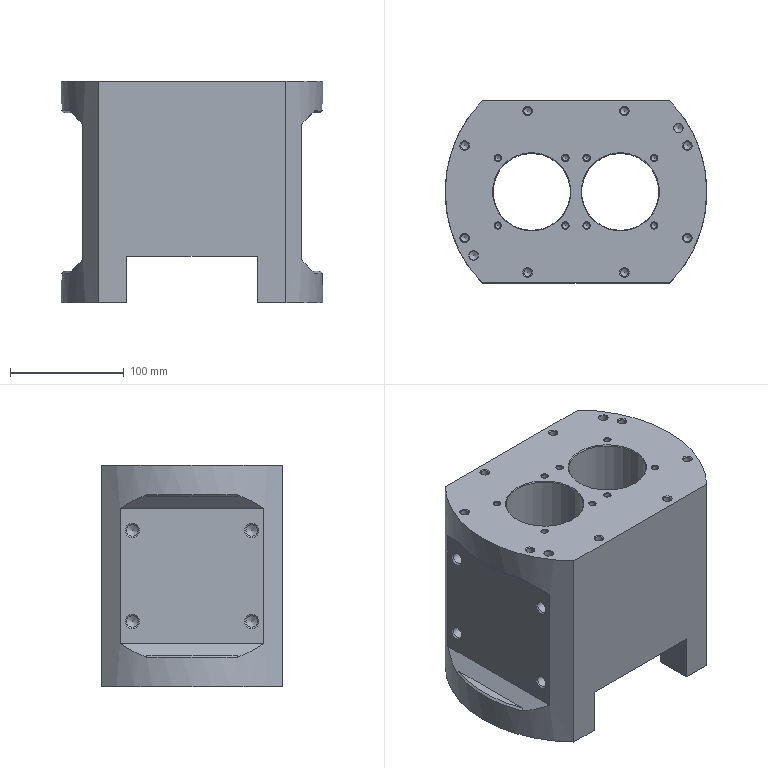NC program | NX | posted with a generic post | part box 230 x 160 x 195 mm
Lines 674 to 1584 of 6546:
(ZLEVEL_PROFILE_COPY , TOOL : D10)
N1340 T10 M6
N1342 G54
N1344 G17 G0 G90 X68.913 Y-34.137 B0. C0. S3500 M3
N1346 G43 Z30. H10
N1348 Z2.859
N1350 G94 G1 Z-0.141 F1000.
N1352 X70.004 Y-33.055
N1354 G3 X70.267 Y-32.09 R1.
N1356 G2 X66.273 Y-7.81 R129.993 F2200.
N1358 X68.051 Y22.092 R121.465
N1360 G1 X68.303 Y23.431
N1362 G2 X70.267 Y32.089 R133.086
N1364 G1 X70.265 Y32.27 Z-0.189
N1366 X70.267 Y32.449 Z-0.236
N1368 X70.272 Y32.628 Z-0.283
N1370 G3 X68.163 Y23.431 R133.781
N1372 G1 X67.911 Y22.092
N1374 G3 X66.131 Y-7.81 R121.38
N1376 X70.272 Y-32.628 R129.905
N1378 G1 X70.27 Y-32.808 Z-0.33
N1380 X70.272 Y-32.987 Z-0.377
N1382 X70.277 Y-33.165 Z-0.424
N1384 G2 X66.381 Y-12.366 R130.972
N1386 X67.074 Y17.919 R119.365
N1388 X70.277 Y33.166 R136.927
N1390 G1 X70.274 Y33.342 Z-0.471
N1392 X70.276 Y33.518 Z-0.519
N1394 X70.279 Y33.693 Z-0.566
N1396 G3 X67.971 Y23.877 R141.858
N1398 G1 X67.884 Y23.431
N1400 G3 X66.093 Y-10.934 R121.273
N1402 X70.279 Y-33.692 R132.524
N1404 G1 X70.281 Y-33.863 Z-0.613
N1406 X70.282 Y-34.033 Z-0.66
N1408 X70.287 Y-34.203 Z-0.707
N1410 G2 X65.995 Y-11.381 R132.113
N1412 X67.744 Y23.431 R121.1
N1414 G1 X67.832 Y23.877
N1416 G2 X70.287 Y34.203 R138.883
N1418 G1 X70.286 Y34.373 Z-0.754
N1420 X70.287 Y34.543 Z-0.801
N1422 X70.293 Y34.711 Z-0.849
N1424 G3 X67.692 Y23.877 R138.715
N1426 G1 X67.604 Y23.431
N1428 G3 X65.941 Y-12.273 R121.022
N1430 X70.293 Y-34.712 R132.842
N1432 G1 X70.29 Y-34.879 Z-0.896
N1434 X70.292 Y-35.044 Z-0.943
N1436 X70.299 Y-35.207 Z-0.99
N1438 G2 X66.233 Y-15.892 R133.312
N1440 X66.849 Y20.049 R119.865
N1442 X70.299 Y35.207 R138.502
N1444 G1 X70.297 Y35.371 Z-1.037
N1446 X70.298 Y35.534 Z-1.084
N1448 X70.305 Y35.695 Z-1.131
N1450 G3 X67.413 Y23.877 R138.622
N1452 G1 X67.324 Y23.431
N1454 G3 X65.66 Y-12.273 R120.9
N1456 X70.305 Y-35.695 R132.646
N1458 G1 X70.302 Y-35.859 Z-1.179
N1460 X70.304 Y-36.022 Z-1.226
N1462 X70.31 Y-36.183 Z-1.273
N1464 G2 X65.771 Y-14.505 R134.113
N1466 X67.184 Y23.431 R120.734
N1468 G1 X67.273 Y23.877
N1470 G2 X70.31 Y36.184 R140.183
N1472 G1 X70.306 Y36.346 Z-1.32
N1474 X70.307 Y36.506 Z-1.367
N1476 X70.315 Y36.665 Z-1.414
N1478 G3 X67.134 Y23.877 R141.731
N1480 G1 X67.044 Y23.431
N1482 G3 X65.74 Y-15.397 R120.755
N1484 X70.315 Y-36.664 R135.262
N1486 G1 X70.313 Y-36.822 Z-1.461
N1488 X70.315 Y-36.98 Z-1.509
N1490 X70.321 Y-37.135 Z-1.556
N1492 G2 X65.6 Y-15.397 R135.399
N1494 X66.651 Y22.092 R120.306
N1496 X70.32 Y37.136 R140.552
N1498 G1 X70.319 Y37.293 Z-1.603
N1500 X70.321 Y37.449 Z-1.65
N1502 X70.326 Y37.604 Z-1.697
N1504 G3 X66.68 Y22.984 R141.925
N1506 X65.46 Y-15.397 R120.284
N1508 X70.326 Y-37.604 R135.836
N1510 G1 X70.324 Y-37.759 Z-1.744
N1512 X70.326 Y-37.913 Z-1.791
N1514 X70.332 Y-38.066 Z-1.839
N1516 G2 X65.908 Y-19.414 R138.626
N1518 X64.474 Y-6.025 R118.166
N1520 X64.4 Y-3.039 R60.156
N1522 G1 Y2.959
N1524 G2 X64.526 Y6.868 R60.811
N1526 G1 X64.644 Y8.703
N1528 X64.674 Y9.149
N1530 G2 X68.118 Y30.125 R126.73
N1532 G1 X68.344 Y31.018
N1534 G2 X70.332 Y38.065 R142.346
N1536 G1 X70.331 Y38.218 Z-1.886
N1538 X70.334 Y38.37 Z-1.933
N1540 X70.338 Y38.521 Z-1.98
N1542 G3 X68.321 Y31.464 R141.46
N1544 G1 X68.206 Y31.018
N1546 G3 X64.533 Y9.149 R127.197
N1548 X64.4 Y6.385 R42.783
N1550 G1 Y-6.39
N1552 G3 X64.48 Y-8.386 R34.933
N1554 X65.768 Y-19.414 R116.791
N1556 X70.339 Y-38.52 R138.489
N1558 G1 Y-38.672 Z-2.028
N1560 X70.341 Y-38.824 Z-2.075
N1562 X70.346 Y-38.974 Z-2.122
N1564 G2 X65.702 Y-19.86 R139.282
N1566 X64.433 Y-9.595 R115.739
N1568 G1 X64.401 Y-8.703
N1570 X64.4 Y-8.533
N1572 Y8.538
N1574 X64.401 Y8.703
N1576 X64.433 Y9.595
N1578 G2 X68.067 Y31.018 R126.18
N1580 G1 X68.184 Y31.464
N1582 G2 X70.345 Y38.976 R147.744
N1584 G1 Y39.129 Z-2.169
N1586 X70.347 Y39.281 Z-2.217
N1588 X70.352 Y39.432 Z-2.264
N1590 G3 X68.522 Y33.249 R155.693
N1592 G1 X68.4 Y32.803
N1594 G3 X64.533 Y12.273 R129.403
N1596 X64.4 Y10.22 R21.989
N1598 G1 Y-10.223
N1600 G3 X64.477 Y-11.687 R17.623
N1602 X65.343 Y-18.521 R108.629
N1604 X70.353 Y-39.429 R139.073
N1606 G1 X70.352 Y-39.58 Z-2.312
N1608 X70.355 Y-39.731 Z-2.359
N1610 X70.36 Y-39.881 Z-2.406
N1612 G2 X65.897 Y-22.538 R143.324
N1614 X64.446 Y-12.719 R116.396
N1616 X64.4 Y-11.707 R14.603
N1618 G1 Y11.702
N1620 G2 X64.466 Y12.906 R10.992
N1622 X67.931 Y31.563 R128.608
N1624 X70.359 Y39.886 R164.25
N1626 G1 Y40.037 Z-2.454
N1628 X70.362 Y40.187 Z-2.501
N1630 X70.367 Y40.337 Z-2.549
N1632 G3 X68.621 Y34.588 R175.228
N1634 G1 X68.494 Y34.142
N1636 G3 X64.616 Y15.397 R131.517
N1638 G1 X64.561 Y14.951
N1640 X64.472 Y14.179
N1642 G3 X64.4 Y13.001 R11.826
N1644 G1 Y-12.998
N1646 G3 X64.486 Y-14.327 R12.592
N1648 X65.928 Y-23.431 R115.814
N1650 X70.369 Y-40.33 R145.407
N1652 G1 Y-40.482 Z-2.596
N1654 X70.372 Y-40.632 Z-2.644
N1656 X70.377 Y-40.781 Z-2.691
N1658 G2 X66.057 Y-24.769 R149.788
N1660 X64.475 Y-15.397 R130.935
N1662 X64.4 Y-14.176 R10.242
N1664 G1 Y14.18
N1666 G2 X64.475 Y15.397 R10.235
N1668 X68.871 Y35.927 R132.708
N1670 G1 X69.002 Y36.373
N1672 X70.246 Y40.39
N1674 X70.375 Y40.79
N1676 X70.376 Y40.947 Z-2.739
N1678 X70.379 Y41.104 Z-2.787
N1680 X70.383 Y41.26 Z-2.834
N1682 G3 X68.367 Y34.657 R234.287
N1684 X64.48 Y16.428 R129.606
N1686 X64.4 Y15.267 R8.433
N1688 G1 Y-15.269
N1690 G3 X64.479 Y-16.414 R8.376
N1692 X67.373 Y-31.018 R127.116
N1694 X70.387 Y-41.249 R177.576
N1696 G1 X70.388 Y-41.407 Z-2.882
N1698 X70.392 Y-41.564 Z-2.929
N1700 X70.396 Y-41.721 Z-2.977
N1702 G2 X68.209 Y-34.588 R250.981
N1704 X64.581 Y-18.138 R132.255
N1706 G1 X64.509 Y-17.629
N1708 G2 X64.4 Y-16.281 R9.712
N1710 G1 Y16.278
N1712 G2 X64.509 Y17.629 R9.699
N1714 G1 X64.581 Y18.136
N1716 G2 X68.73 Y36.373 R134.02
N1718 G1 X68.998 Y37.266
N1720 X70.253 Y41.282
N1722 X70.392 Y41.733
N1724 X70.329 Y41.761 Z-3.049
N1726 X70.249 Y41.798 Z-3.12
N1728 G2 X70.122 Y41.283 R4.325
N1730 G1 X68.862 Y37.266
N1732 X68.593 Y36.373
N1734 G3 X64.5 Y18.521 R133.997
N1736 X64.4 Y17.233 R8.601
N1738 G1 Y-17.237
N1740 G3 X64.5 Y-18.521 R8.595
N1742 X66.326 Y-27.894 R132.186
N1744 X70.067 Y-41.09 R159.82
N1746 G2 X70.245 Y-41.805 R4.982
N1748 G1 X70.142 Y-41.745 Z-3.192
N1750 X70.058 Y-41.683 Z-3.263
N1752 G3 X70.02 Y-41.389 R0.813
N1754 G2 X67.665 Y-33.637 R209.296
N1756 X64.508 Y-19.412 R127.619
N1758 X64.4 Y-18.142 R8.332
N1760 G1 Y18.139
N1762 G2 X64.508 Y19.414 R8.331
N1764 X68.456 Y36.373 R132.204
N1766 G1 X68.725 Y37.266
N1768 X70.017 Y41.386
N1770 G3 X70.06 Y41.694 R0.952
N1772 G1 X70.032 Y41.864 Z-3.299
N1774 X69.998 Y42.034 Z-3.335
N1776 X69.974 Y42.203 Z-3.371
N1778 X69.95 Y42.373 Z-3.407
N1780 G3 X69.904 Y41.506 R6.558
N1782 G1 X69.85 Y41.282
N1784 X69.145 Y39.051
N1786 X69.006 Y38.605
N1788 X68.727 Y37.712
N1790 G3 X64.665 Y21.199 R136.391
N1792 G1 X64.516 Y20.307
N1794 G3 X64.4 Y18.968 R8.213
N1796 G1 Y-18.968
N1798 G3 X64.516 Y-20.307 R8.213
N1800 G1 X64.665 Y-21.199
N1802 G3 X68.846 Y-38.106 R137.693
N1804 G1 X69.849 Y-41.282
N1806 X69.904 Y-41.506
N1808 G3 X69.947 Y-42.376 R5.8
N1810 G1 X69.866 Y-42.518 Z-3.479
N1812 X69.794 Y-42.658 Z-3.55
N1814 X69.789 Y-42.621
N1816 X69.76 Y-41.506
N1818 X69.712 Y-41.282
N1820 X68.479 Y-37.331
N1822 G2 X65.703 Y-27.001 R134.232
N1824 X64.532 Y-21.24 R132.357
N1826 X64.4 Y-19.826 R8.335
N1828 G1 Y19.825
N1830 G2 X64.538 Y21.282 R8.569
N1832 X68.696 Y38.055 R137.191
N1834 G1 X69.723 Y41.305
N1836 X69.756 Y41.399
N1838 Y41.499
N1840 X69.797 Y42.655
N1842 X69.721 Y42.793 Z-3.622
N1844 X69.655 Y42.931 Z-3.693
N1846 X69.62 Y41.541
N1848 G2 X69.571 Y41.246 R1.058
N1850 G1 X68.872 Y39.051
N1852 X68.328 Y37.303
N1854 G3 X64.533 Y21.989 R133.678
N1856 X64.4 Y20.614 R7.933
N1858 G1 Y-20.614
N1860 G3 X64.529 Y-21.966 R7.931
N1862 X66.732 Y-31.746 R123.326
N1864 X69.533 Y-41.126 R175.566
N1866 G2 X69.616 Y-41.607 R1.674
N1868 G1 X69.65 Y-42.936
N1870 X69.571 Y-43.071 Z-3.765
N1872 X69.506 Y-43.205 Z-3.836
N1874 G3 X69.443 Y-41.282 R34.087
N1876 G2 X67.162 Y-33.815 R211.646
N1878 X64.536 Y-22.731 R125.863
N1880 X64.4 Y-21.354 R7.816
N1882 G1 Y21.353
N1884 G2 X64.55 Y22.799 R7.816
N1886 X68.041 Y36.82 R132.86
N1888 G1 X68.177 Y37.266
N1890 X69.164 Y40.39
N1892 X69.439 Y41.254
N1894 G3 X69.478 Y41.493 R0.837
N1896 G1 X69.504 Y43.068
N1898 X69.512 Y43.2
N1900 X69.433 Y43.332 Z-3.907
N1902 X69.366 Y43.463 Z-3.979
N1904 X69.334 Y41.473
N1906 X69.338 Y41.376
N1908 X69.313 Y41.282
N1910 X68.245 Y37.91
N1912 G3 X64.578 Y23.68 R134.741
N1914 X64.4 Y22.092 R9.31
N1916 G1 Y-22.092
N1918 G3 X64.567 Y-23.624 R8.839
N1920 X67.308 Y-34.803 R129.797
N1922 X69.308 Y-41.282 R230.906
N1924 G2 X69.359 Y-43.47 R51.569
N1926 G1 X69.286 Y-43.608 Z-4.05
N1928 X69.221 Y-43.747 Z-4.121
N1930 X69.215 Y-43.514
N1932 X69.192 Y-41.506
N1934 X69.173 Y-41.282
N1936 G2 X67.249 Y-35.071 R238.178
N1938 X64.535 Y-24.155 R130.185
N1940 X64.4 Y-22.808 R6.766
N1942 G1 Y22.805
N1944 G2 X64.541 Y24.194 R6.911
N1946 X68.123 Y37.954 R135.777
N1948 G1 X69.179 Y41.282
N1950 X69.196 Y41.506
N1952 X69.222 Y43.514
N1954 X69.228 Y43.738
N1956 X69.157 Y43.897 Z-4.191
N1958 X69.089 Y44.055 Z-4.262
N1960 X69.086 Y43.96
N1962 X69.056 Y41.506
N1964 X69.044 Y41.282
N1966 X67.968 Y37.89
N1968 G3 X64.54 Y24.839 R133.943
N1970 X64.4 Y23.484 R6.611
N1972 G1 Y-23.486
N1974 G3 X64.538 Y-24.829 R6.594
N1976 X67.047 Y-34.845 R127.775
N1978 X69.038 Y-41.282 R236.882
N1980 G1 X69.051 Y-41.506
N1982 X69.079 Y-43.96
N1984 X69.082 Y-44.064
N1986 X69.011 Y-44.243 Z-4.333
N1988 X68.943 Y-44.421 Z-4.404
N1990 X68.939 Y-43.96
N1992 X68.91 Y-41.506
N1994 X68.903 Y-41.282
N1996 G2 X67.347 Y-36.315 R363.413
N1998 X64.559 Y-25.562 R129.331
N2000 X64.4 Y-24.137 R7.216
N2002 G1 Y24.138
N2004 G2 X64.561 Y25.571 R7.217
N2006 X67.954 Y38.286 R134.904
N2008 G1 X68.813 Y40.974
N2010 X68.909 Y41.282
N2012 X68.916 Y41.506
N2014 X68.945 Y43.96
N2016 X68.948 Y44.414
N2018 X68.878 Y44.594 Z-4.474
N2020 X68.809 Y44.773 Z-4.545
N2022 X68.807 Y44.407
N2024 X68.773 Y41.282
N2026 X68.637 Y40.836
N2028 X67.774 Y38.149
N2030 G3 X64.541 Y26.108 R128.966
N2032 X64.4 Y24.769 R7.655
N2034 G1 Y-24.769
N2036 G3 X64.569 Y-26.239 R7.46
N2038 G1 X64.735 Y-27.001
N2040 G3 X67.36 Y-36.82 R137.507
N2042 G1 X67.499 Y-37.266
N2044 X68.632 Y-40.836
N2046 X68.767 Y-41.282
N2048 X68.805 Y-44.778
N2050 X68.736 Y-44.955 Z-4.616
N2052 X68.67 Y-45.132 Z-4.686
N2054 X68.626 Y-41.282
N2056 X68.498 Y-40.836
N2058 X67.784 Y-38.605
N2060 G2 X64.598 Y-27.001 R139.858
N2062 X64.4 Y-25.401 R7.301
N2064 G1 Y25.399
N2066 G2 X64.598 Y27.001 R7.299
N2068 X67.922 Y39.028 R139.65
N2070 G1 X68.504 Y40.836
N2072 X68.633 Y41.282
N2074 X68.673 Y45.129
N2076 X68.599 Y45.305 Z-4.757
N2078 X68.533 Y45.481 Z-4.828
N2080 X68.493 Y41.282
N2082 G2 X68.335 Y40.724 R7.93
N2084 G1 X67.922 Y39.443
N2086 G3 X64.561 Y27.447 R141.207
N2088 X64.4 Y26.006 R6.468
N2090 G1 Y-26.006
N2092 G3 X64.569 Y-27.482 R6.465
N2094 X67.725 Y-38.848 R142.365
N2096 G1 X68.293 Y-40.606
N2098 G2 X68.486 Y-41.282 R10.277
N2100 G1 X68.531 Y-45.483
N2102 X68.456 Y-45.657 Z-4.899
N2104 X68.389 Y-45.831 Z-4.969
N2106 X68.346 Y-41.282
N2108 X68.302 Y-41.059
N2110 X67.359 Y-38.109
N2112 G2 X64.585 Y-28.109 R134.184
N2114 X64.4 Y-26.598 R6.925
N2116 G1 Y26.6
N2118 G2 X64.578 Y28.081 R6.924
N2120 X68.096 Y40.39 R141.405
N2122 G1 X68.325 Y41.106
N2124 X68.355 Y41.192
N2126 X68.353 Y41.282
N2128 X68.39 Y45.83
N2130 X68.317 Y46.004 Z-5.04
N2132 X68.247 Y46.178 Z-5.111
N2134 X68.213 Y41.308
N2136 G2 X68.169 Y41.031 R0.928
N2138 G1 X67.963 Y40.39
N2140 G3 X64.578 Y28.644 R139.644
N2142 X64.4 Y27.176 R6.636
N2144 G1 Y-27.169
N2146 G3 X64.578 Y-28.644 R6.635
N2148 X68.039 Y-40.646 R145.378
N2150 G2 X68.207 Y-41.282 R4.919
N2152 X68.246 Y-46.179 R255.457
N2154 G1 X68.175 Y-46.353 Z-5.181
N2156 X68.11 Y-46.526 Z-5.252
N2158 G3 X68.067 Y-41.282 R363.385
N2160 G1 X68.033 Y-41.059
N2162 G2 X65.393 Y-32.357 R174.697
N2164 X64.578 Y-29.206 R94.72
N2166 X64.4 Y-27.743 R6.759
N2168 G1 Y27.744
N2170 G2 X64.578 Y29.206 R6.759
N2172 X68. Y40.904 R141.457
N2174 G3 X68.073 Y41.337 R1.376
N2176 G1 X68.111 Y46.526
N2178 X68.035 Y46.696 Z-5.323
N2180 X67.969 Y46.866 Z-5.394
N2182 X67.943 Y42.175
N2184 X67.932 Y41.244
N2186 G2 X67.883 Y40.96 R0.919
N2188 G3 X64.624 Y29.964 R148.891
N2190 X64.4 Y28.297 R7.242
N2192 G1 Y-28.297
N2194 G3 X64.618 Y-29.941 R7.175
N2196 X66.848 Y-37.768 R135.985
N2198 G1 X67.922 Y-41.149
N2200 G2 X67.968 Y-46.866 R278.812
N2202 G1 X67.893 Y-47.035 Z-5.464
N2204 X67.827 Y-47.203 Z-5.535
N2206 G3 X67.791 Y-41.251 R423.014
N2208 X67.747 Y-40.994 R0.847
N2210 G2 X64.578 Y-30.319 R161.459
N2212 X64.4 Y-28.841 R6.285
N2214 G1 Y28.838
N2216 G2 X64.578 Y30.319 R6.283
N2218 X67.778 Y41.059 R153.85
N2220 G1 X67.793 Y41.282
N2222 X67.823 Y46.638
N2224 X67.827 Y47.202
N2226 X67.752 Y47.37 Z-5.606
N2228 X67.682 Y47.539 Z-5.676
N2230 Y46.638
N2232 X67.654 Y41.282
N2234 X67.645 Y41.059
N2236 G3 X64.578 Y30.83 R153.623
N2238 X64.4 Y29.373 R6.519
N2240 G1 Y-29.37
N2242 G3 X64.578 Y-30.83 R6.518
N2244 X67.619 Y-41.011 R160.641
N2246 G2 X67.653 Y-41.212 R0.659
N2248 X67.682 Y-47.539 R419.652
N2250 G1 X67.611 Y-47.707 Z-5.747
N2252 X67.544 Y-47.876 Z-5.818
N2254 X67.531 Y-42.621
N2256 X67.516 Y-41.282
N2258 X67.502 Y-41.059
N2260 G2 X64.612 Y-31.464 R158.472
N2262 X64.4 Y-29.881 R6.343
N2264 G1 Y29.881
N2266 G2 X64.612 Y31.464 R6.343
N2268 X67.511 Y41.059 R151.278
N2270 G3 X67.544 Y47.875 R594.075
N2272 G1 X67.47 Y48.041 Z-5.889
N2274 X67.403 Y48.206 Z-5.959
N2276 X67.384 Y42.175
N2278 X67.373 Y41.059
N2280 X67.162 Y40.39
N2282 G3 X64.596 Y31.91 R136.704
N2284 X64.4 Y30.405 R6.491
N2286 G1 Y-30.405
N2288 G3 X64.596 Y-31.91 R6.492
N2290 X67.368 Y-41.059 R160.295
N2292 G1 X67.379 Y-41.282
N2294 X67.403 Y-48.206
N2296 X67.328 Y-48.369 Z-6.03
N2298 X67.261 Y-48.531 Z-6.101
N2300 X67.246 Y-41.729
N2302 X67.234 Y-41.059
N2304 G2 X64.699 Y-32.803 R175.194
N2306 G1 X64.578 Y-32.35
N2308 G2 X64.4 Y-30.906 R6.61
N2310 G1 Y30.906
N2312 G2 X64.578 Y32.35 R6.61
N2314 G1 X64.699 Y32.803
N2316 G2 X67.179 Y40.836 R144.311
N2318 G1 X67.234 Y41.059
N2320 X67.244 Y42.175
N2322 X67.261 Y48.531
N2324 X67.187 Y48.693 Z-6.171
N2326 X67.117 Y48.856 Z-6.242
N2328 X67.105 Y42.175
N2330 X67.094 Y41.059
N2332 X67.046 Y40.836
N2334 G3 X64.684 Y33.249 R149.366
N2336 X64.4 Y31.401 R6.721
N2338 G1 Y-31.403
N2340 G3 X64.684 Y-33.249 R6.723
N2342 X67.1 Y-41.059 R192.176
N2344 G1 X67.108 Y-41.729
N2346 X67.117 Y-48.856
N2348 X67.046 Y-49.018 Z-6.313
N2350 X66.977 Y-49.181 Z-6.384
N2352 X66.969 Y-41.729
N2354 X66.964 Y-41.059
N2356 X66.904 Y-40.836
N2358 X66.607 Y-39.944
N2360 G2 X64.624 Y-33.501 R150.722
N2362 X64.4 Y-31.89 R5.908
N2364 G1 Y31.89
N2366 G2 X64.622 Y33.495 R5.902
N2368 X66.912 Y40.836 R142.669
N2370 G1 X66.955 Y41.059
N2372 X66.965 Y42.175
N2374 X66.977 Y49.18
N2376 X66.904 Y49.341 Z-6.454
N2378 X66.84 Y49.501 Z-6.525
N2380 X66.834 Y49.316
N2382 X66.821 Y41.207
N2384 G2 X66.778 Y40.836 R1.645
N2386 G3 X64.661 Y34.112 R143.8
N2388 X64.4 Y32.357 R6.68
N2390 G1 Y-32.357
N2392 G3 X64.578 Y-33.798 R6.667
N2394 X66.691 Y-40.584 R137.913
N2396 G2 X66.825 Y-41.059 R4.753
N2398 G1 X66.84 Y-49.501
N2400 X66.763 Y-49.66 Z-6.596
N2402 X66.695 Y-49.819 Z-6.666
N2404 X66.687 Y-41.103
N2406 G3 X66.642 Y-40.831 R0.84
N2408 G2 X64.671 Y-34.588 R136.317
N2410 X64.4 Y-32.834 R6.319
N2412 G1 Y32.835
N2414 G2 X64.671 Y34.588 R6.318
N2416 X66.645 Y40.836 R133.395
N2418 G3 X66.682 Y41.177 R1.599
N2420 G1 X66.695 Y49.819
N2422 X66.621 Y49.976 Z-6.737
N2424 X66.552 Y50.132 Z-6.808
N2426 X66.537 Y40.943
N2428 X66.526 Y40.889
N2430 G3 X64.667 Y35.034 R137.959
N2432 X64.4 Y33.297 R6.318
N2434 G1 Y-33.298
N2436 G3 X64.667 Y-35.034 R6.318
N2438 X66.541 Y-40.941 R146.081
N2440 G1 X66.548 Y-41.
N2442 X66.552 Y-50.132
N2444 X66.48 Y-50.289 Z-6.879
N2446 X66.415 Y-50.446 Z-6.949
N2448 X66.409 Y-50.208
N2450 X66.405 Y-40.971
N2452 X66.402 Y-40.915
N2454 G2 X64.663 Y-35.481 R148.465
N2456 X64.4 Y-33.753 R6.314
N2458 G1 Y33.755
N2460 G2 X64.663 Y35.481 R6.314
N2462 X66.396 Y40.917 R172.222
N2464 G1 X66.403 Y41.729
N2466 X66.409 Y50.208
N2468 X66.415 Y50.446
N2470 X66.339 Y50.602 Z-7.02
N2472 X66.272 Y50.758 Z-7.091
N2474 X66.263 Y41.729
N2476 X66.26 Y40.946
N2478 X66.245 Y40.836
N2480 G3 X64.659 Y35.927 R148.881
N2482 X64.4 Y34.202 R6.309
N2484 G1 Y-34.202
N2486 G3 X64.659 Y-35.927 R6.309
N2488 X66.094 Y-40.39 R143.354
N2490 G1 X66.245 Y-40.836
N2492 X66.266 Y-40.945
N2494 X66.268 Y-50.655
N2496 X66.271 Y-50.758
N2498 X66.197 Y-50.913 Z-7.161
N2500 X66.127 Y-51.068 Z-7.232
N2502 X66.125 Y-41.282
N2504 X66.124 Y-40.919
N2506 X66.112 Y-40.836
N2508 G2 X64.661 Y-36.373 R149.181
N2510 X64.4 Y-34.646 R5.989
N2512 G1 Y34.647
N2514 G2 X64.661 Y36.373 R5.989
N2516 X66.112 Y40.836 R149.18
N2518 G1 X66.121 Y40.924
N2520 X66.127 Y51.068
N2522 X66.056 Y51.22 Z-7.303
N2524 X65.99 Y51.371 Z-7.373
N2526 X65.979 Y40.836
N2528 G3 X64.669 Y36.82 R133.798
N2530 X64.4 Y35.081 R6.086
N2532 G1 Y-35.082
N2534 G3 X64.669 Y-36.82 R6.088
N2536 X65.979 Y-40.836 R132.601
N2538 G1 X65.99 Y-51.371
N2540 X65.914 Y-51.523 Z-7.444
N2542 X65.847 Y-51.674 Z-7.515
N2544 X65.844 Y-51.547
N2546 Y-41.074
N2548 Y-40.826
N2550 G2 X64.677 Y-37.266 R116.391
N2552 X64.4 Y-35.513 R6.095
N2554 G1 Y35.515
N2556 G2 X64.677 Y37.266 R6.097
N2558 X65.844 Y40.818 R104.557
N2560 G1 Y41.073
N2562 X65.841 Y42.175
N2564 X65.844 Y51.547
N2566 X65.847 Y51.674
N2568 X65.773 Y51.826 Z-7.586
N2570 X65.703 Y51.977 Z-7.656
N2572 X65.701 Y42.175
N2574 X65.702 Y41.443
N2576 Y40.801
N2578 G3 X64.685 Y37.712 R102.699
N2580 X64.4 Y35.927 R6.081
N2582 G1 Y-35.927
N2584 G3 X64.685 Y-37.712 R6.081
N2586 X65.702 Y-40.801 R102.75
N2588 G1 Y-41.443
N2590 X65.703 Y-51.977
N2592 X65.632 Y-52.128 Z-7.727
N2594 X65.565 Y-52.279 Z-7.798
N2596 X65.561 Y-51.994
N2598 X65.559 Y-41.809
N2600 X65.561 Y-41.729
N2602 Y-40.783
N2604 X64.835 Y-38.605
N2606 X64.693 Y-38.158
N2608 G2 X64.4 Y-36.358 R6.096
N2610 G1 Y36.359
N2612 G2 X64.693 Y38.158 R6.098
N2614 G1 X64.835 Y38.605
N2616 X65.561 Y40.783
N2618 Y41.729
N2620 X65.559 Y41.809
N2622 X65.561 Y51.994
N2624 X65.565 Y52.278
N2626 X65.49 Y52.427 Z-7.868
N2628 X65.423 Y52.576 Z-7.939
N2630 X65.419 Y52.44
N2632 Y41.729
N2634 Y40.757
N2636 X64.701 Y38.605
N2638 G3 X64.4 Y36.771 R6.061
N2640 G1 Y-36.771
N2642 G3 X64.701 Y-38.605 R6.061
N2644 G1 X65.419 Y-40.757
N2646 Y-41.729
N2648 Y-52.44
N2650 X65.423 Y-52.576
N2652 X65.349 Y-52.722 Z-8.01
N2654 X65.279 Y-52.869 Z-8.081
N2656 X65.278 Y-42.524
N2658 Y-40.731
N2660 G2 X64.578 Y-38.609 R31.247
N2662 X64.4 Y-37.181 R6.257
N2664 G1 Y37.182
N2666 G2 X64.578 Y38.609 R6.258
N2668 X65.278 Y40.731 R31.247
N2670 G1 Y42.524
N2672 X65.279 Y52.869
N2674 X65.207 Y53.015 Z-8.151
N2676 X65.14 Y53.162 Z-8.222
N2678 X65.137 Y52.886
N2680 X65.135 Y42.879
N2682 X65.137 Y42.621
N2684 X65.136 Y40.694
N2686 X64.729 Y39.497
N2688 G3 X64.4 Y37.584 R5.738
N2690 G1 Y-37.584
N2692 G3 X64.729 Y-39.497 R5.738
N2694 G1 X65.136 Y-40.694
N2696 X65.137 Y-42.621
N2698 Y-52.886
N2700 X65.14 Y-53.162
N2702 X65.066 Y-53.308 Z-8.293
N2704 X64.998 Y-53.454 Z-8.363
N2706 X64.995 Y-53.333
N2708 Y-43.068
N2710 Y-40.679
N2712 X64.578 Y-39.395
N2714 G2 X64.4 Y-37.984 R6.257
N2716 G1 Y37.985
N2718 G2 X64.578 Y39.395 R6.257
N2720 G1 X64.995 Y40.679
N2722 Y43.068
N2724 Y53.333
N2726 X64.998 Y53.454
N2728 X64.924 Y53.601 Z-8.434
N2730 X64.855 Y53.747 Z-8.505
N2732 X64.854 Y43.514
N2734 Y40.653
N2736 X64.625 Y39.944
N2738 G3 X64.4 Y38.392 R5.46
N2740 G1 Y-38.379
N2742 G3 X64.656 Y-40.03 R5.454
N2744 G1 X64.854 Y-40.653
N2746 Y-43.514
N2748 X64.855 Y-53.747
N2750 X64.783 Y-53.89 Z-8.576
N2752 X64.716 Y-54.032 Z-8.646
N2754 X64.712 Y-53.779
N2756 Y-43.92
N2758 Y-40.619
N2760 G2 X64.4 Y-38.769 R5.978
N2762 G1 Y38.769
N2764 G2 X64.712 Y40.619 R5.978
N2766 G1 Y43.92
N2768 Y53.779
N2770 X64.716 Y54.032
N2772 X64.642 Y54.174 Z-8.717
N2774 X64.574 Y54.316 Z-8.788
N2776 X64.571 Y54.225
N2778 Y43.96
N2780 Y40.543
N2782 G3 X64.4 Y39.154 R6.444
N2784 G1 Y-39.154
N2786 G3 X64.571 Y-40.543 R6.444
N2788 G1 Y-43.96
N2790 Y-54.225
N2792 X64.574 Y-54.316
N2794 X64.5 Y-54.457 Z-8.858
N2796 X64.432 Y-54.599 Z-8.929
N2798 X64.429 Y-44.407
N2800 Y-40.145
N2802 X64.4 Y-39.536
N2804 Y39.536
N2806 X64.429 Y40.145
N2808 Y44.407
N2810 X64.432 Y54.599
N2812 X64.359 Y54.741 Z-9.
N2814 X64.292 Y54.882 Z-9.071
N2816 X64.288 Y54.671
N2818 Y44.853
N2820 Y-44.853
N2822 Y-54.671
N2824 X64.292 Y-54.882
N2826 X64.217 Y-55.023 Z-9.141
N2828 X64.148 Y-55.164 Z-9.212
N2830 X64.147 Y-55.118
N2832 Y-45.266
N2834 Y45.266
N2836 Y55.118
N2838 X64.148 Y55.164
N2840 X64.076 Y55.302 Z-9.283
N2842 X64.008 Y55.441 Z-9.353
N2844 X64.005 Y55.118
N2846 Y45.299
N2848 Y-45.299
N2850 Y-55.118
N2852 X64.008 Y-55.441
N2854 X63.934 Y-55.578 Z-9.424
N2856 X63.867 Y-55.716 Z-9.495
N2858 X63.864 Y-55.564
N2860 Y-45.745
N2862 Y45.745
N2864 Y55.564
N2866 X63.867 Y55.716
N2868 X63.793 Y55.853 Z-9.566
N2870 X63.723 Y55.99 Z-9.636
N2872 X63.722 Y46.192
N2874 Y-46.192
N2876 X63.723 Y-55.99
N2878 X63.652 Y-56.127 Z-9.707
N2880 X63.585 Y-56.264 Z-9.778
N2882 X63.581 Y-56.01
N2884 Y-46.192
N2886 Y56.01
N2888 X63.585 Y56.264
N2890 X63.51 Y56.401 Z-9.848
N2892 X63.442 Y56.538 Z-9.919
N2894 X63.439 Y56.457
N2896 X63.438 Y46.883
N2898 X63.439 Y46.638
N2900 Y-46.638
N2902 X63.438 Y-46.883
N2904 X63.439 Y-56.457
N2906 X63.442 Y-56.538
N2908 X63.369 Y-56.672 Z-9.99
N2910 X63.301 Y-56.806 Z-10.061
N2912 X63.298 Y-56.457
N2914 Y56.457
N2916 X63.301 Y56.806
N2918 X63.227 Y56.939 Z-10.131
N2920 X63.161 Y57.072 Z-10.202
N2922 X63.157 Y56.903
N2924 Y-56.903
N2926 X63.161 Y-57.072
N2928 X63.086 Y-57.205 Z-10.273
N2930 X63.015 Y-57.338 Z-10.343
N2932 Y-47.531
N2934 Y47.531
N2936 Y57.338
N2938 X62.945 Y57.471 Z-10.414
N2940 X62.878 Y57.604 Z-10.485
N2942 X62.874 Y57.349
N2944 Y-57.349
N2946 X62.878 Y-57.604
N2948 X62.803 Y-57.737 Z-10.555
N2950 X62.735 Y-57.869 Z-10.626
N2952 X62.732 Y-57.795
N2954 Y57.795
N2956 X62.735 Y57.869
N2958 X62.662 Y58. Z-10.697
N2960 X62.593 Y58.131 Z-10.768
N2962 X62.591 Y48.423
N2964 Y-48.423
N2966 X62.593 Y-58.131
N2968 X62.52 Y-58.26 Z-10.838
N2970 X62.454 Y-58.389 Z-10.909
N2972 X62.45 Y-58.242
N2974 Y58.242
N2976 X62.454 Y58.389
N2978 X62.379 Y58.518 Z-10.98
N2980 X62.31 Y58.647 Z-11.05
N2982 X62.308 Y58.242
N2984 Y-58.242
N2986 X62.31 Y-58.647
N2988 X62.237 Y-58.775 Z-11.121
N2990 X62.17 Y-58.904 Z-11.192
N2992 X62.167 Y-58.688
N2994 Y58.688
N2996 X62.17 Y58.904
N2998 X62.096 Y59.033 Z-11.263
N3000 X62.027 Y59.161 Z-11.333
N3002 X62.025 Y49.762
N3004 Y-49.762
N3006 X62.027 Y-59.161
N3008 X61.955 Y-59.288 Z-11.404
N3010 X61.889 Y-59.415 Z-11.475
N3012 X61.884 Y-59.134
N3014 Y59.134
N3016 X61.889 Y59.415
N3018 X61.813 Y59.542 Z-11.545
N3020 X61.745 Y59.668 Z-11.616
N3022 X61.742 Y59.581
N3024 Y-59.581
N3026 X61.745 Y-59.668
N3028 X61.672 Y-59.793 Z-11.687
N3030 X61.603 Y-59.918 Z-11.758
N3032 X61.601 Y-59.581
N3034 Y59.581
N3036 X61.603 Y59.918
N3038 X61.53 Y60.043 Z-11.828
N3040 X61.465 Y60.167 Z-11.899
N3042 X61.46 Y60.027
N3044 Y-60.027
N3046 X61.465 Y-60.167
N3048 X61.389 Y-60.293 Z-11.97
N3050 X61.321 Y-60.417 Z-12.04
N3052 X61.318 Y-60.027
N3054 Y60.027
N3056 X61.321 Y60.417
N3058 X61.247 Y60.542 Z-12.111
N3060 X61.18 Y60.666 Z-12.182
N3062 X61.177 Y60.473
N3064 Y-60.473
N3066 X61.18 Y-60.666
N3068 X61.106 Y-60.789 Z-12.253
N3070 X61.036 Y-60.912 Z-12.323
N3072 X61.035 Y-51.547
N3074 Y51.547
N3076 X61.036 Y60.912
N3078 X60.965 Y61.033 Z-12.394
N3080 X60.898 Y61.154 Z-12.465
N3082 X60.894 Y60.92
N3084 X60.893 Y52.213
N3086 X60.894 Y51.994
N3088 Y-60.92
N3090 X60.898 Y-61.154
N3092 X60.823 Y-61.276 Z-12.535
N3094 X60.754 Y-61.397 Z-12.606
N3096 X60.752 Y-52.44
N3098 Y52.44
N3100 X60.754 Y61.397
N3102 X60.682 Y61.518 Z-12.677
N3104 X60.616 Y61.639 Z-12.748
N3106 X60.611 Y61.366
N3108 Y-61.366
N3110 X60.616 Y-61.639
N3112 X60.54 Y-61.76 Z-12.818
N3114 X60.473 Y-61.881 Z-12.889
N3116 X60.47 Y-61.812
N3118 Y61.812
N3120 X60.473 Y61.881
N3122 X60.399 Y62.002 Z-12.96
N3124 X60.33 Y62.123 Z-13.03
N3126 X60.328 Y61.812
N3128 Y-61.812
N3130 X60.33 Y-62.123
N3132 X60.258 Y-62.241 Z-13.101
N3134 X60.191 Y-62.359 Z-13.172
N3136 X60.187 Y-62.258
N3138 Y62.258
N3140 X60.191 Y62.359
N3142 X60.116 Y62.476 Z-13.242
N3144 X60.05 Y62.594 Z-13.313
N3146 X60.045 Y62.258
N3148 Y-62.258
N3150 X60.05 Y-62.594
N3152 X59.975 Y-62.712 Z-13.384
N3154 X59.907 Y-62.829 Z-13.455